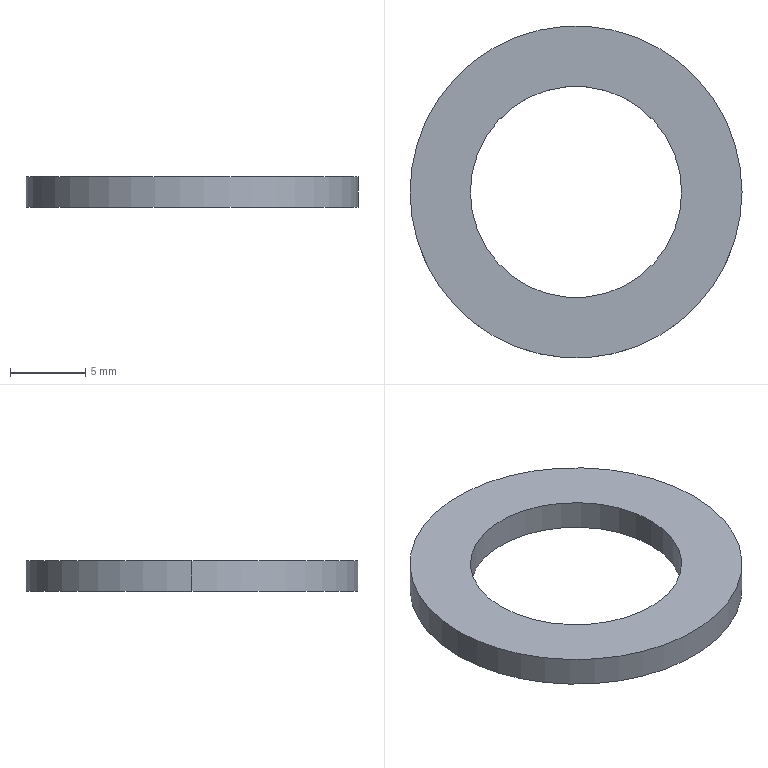Part | SolidWorks | features Extrusion 1 | 1 solid | 6 faces | box 22 x 22 x 2 mm | volume 452.389 mm3 | cylinder 4 | plane 2 | commonest cylinder face diameters 14 x2 22 x2
STEP:
#1=CARTESIAN_POINT('',(-7.,0.,2.));
#2=VERTEX_POINT('',#1);
#3=CARTESIAN_POINT('',(7.,0.,2.));
#4=VERTEX_POINT('',#3);
#5=CARTESIAN_POINT('',(0.,0.,2.));
#6=DIRECTION('',(0.,0.,1.));
#7=DIRECTION('',(1.,0.,0.));
#8=AXIS2_PLACEMENT_3D('',#5,#6,#7);
#9=CIRCLE('',#8,7.);
#10=EDGE_CURVE('',#2,#4,#9,.T.);
#11=ORIENTED_EDGE('',*,*,#10,.T.);
#12=CARTESIAN_POINT('',(7.,0.,0.));
#13=VERTEX_POINT('',#12);
#14=CARTESIAN_POINT('',(7.,0.,2.));
#15=DIRECTION('',(0.,0.,-1.));
#16=VECTOR('',#15,1000.);
#17=LINE('',#14,#16);
#18=EDGE_CURVE('',#4,#13,#17,.T.);
#19=ORIENTED_EDGE('',*,*,#18,.T.);
#20=CARTESIAN_POINT('',(-7.,0.,0.));
#21=VERTEX_POINT('',#20);
#22=CARTESIAN_POINT('',(0.,0.,0.));
#23=DIRECTION('',(0.,0.,1.));
#24=DIRECTION('',(1.,0.,0.));
#25=AXIS2_PLACEMENT_3D('',#22,#23,#24);
#26=CIRCLE('',#25,7.);
#27=EDGE_CURVE('',#21,#13,#26,.T.);
#28=ORIENTED_EDGE('',*,*,#27,.F.);
#29=CARTESIAN_POINT('',(-7.,0.,2.));
#30=DIRECTION('',(0.,0.,-1.));
#31=VECTOR('',#30,1000.);
#32=LINE('',#29,#31);
#33=EDGE_CURVE('',#2,#21,#32,.T.);
#34=ORIENTED_EDGE('',*,*,#33,.F.);
#35=EDGE_LOOP('',(#11,#19,#28,#34));
#36=FACE_OUTER_BOUND('',#35,.T.);
#37=CARTESIAN_POINT('',(0.,0.,2.));
#38=DIRECTION('',(0.,0.,-1.));
#39=DIRECTION('',(-1.,0.,0.));
#40=AXIS2_PLACEMENT_3D('',#37,#38,#39);
#41=CYLINDRICAL_SURFACE('',#40,7.);
#42=ADVANCED_FACE('',(#36),#41,.F.);
#43=CARTESIAN_POINT('',(11.,0.,2.));
#44=VERTEX_POINT('',#43);
#45=CARTESIAN_POINT('',(-11.,0.,2.));
#46=VERTEX_POINT('',#45);
#47=CARTESIAN_POINT('',(0.,0.,2.));
#48=DIRECTION('',(0.,0.,1.));
#49=DIRECTION('',(1.,0.,0.));
#50=AXIS2_PLACEMENT_3D('',#47,#48,#49);
#51=CIRCLE('',#50,11.);
#52=EDGE_CURVE('',#44,#46,#51,.T.);
#53=ORIENTED_EDGE('',*,*,#52,.F.);
#54=CARTESIAN_POINT('',(11.,0.,0.));
#55=VERTEX_POINT('',#54);
#56=CARTESIAN_POINT('',(11.,0.,2.));
#57=DIRECTION('',(0.,0.,-1.));
#58=VECTOR('',#57,1000.);
#59=LINE('',#56,#58);
#60=EDGE_CURVE('',#44,#55,#59,.T.);
#61=ORIENTED_EDGE('',*,*,#60,.T.);
#62=CARTESIAN_POINT('',(-11.,0.,0.));
#63=VERTEX_POINT('',#62);
#64=CARTESIAN_POINT('',(0.,0.,0.));
#65=DIRECTION('',(0.,0.,1.));
#66=DIRECTION('',(1.,0.,0.));
#67=AXIS2_PLACEMENT_3D('',#64,#65,#66);
#68=CIRCLE('',#67,11.);
#69=EDGE_CURVE('',#55,#63,#68,.T.);
#70=ORIENTED_EDGE('',*,*,#69,.T.);
#71=CARTESIAN_POINT('',(-11.,0.,2.));
#72=DIRECTION('',(0.,0.,-1.));
#73=VECTOR('',#72,1000.);
#74=LINE('',#71,#73);
#75=EDGE_CURVE('',#46,#63,#74,.T.);
#76=ORIENTED_EDGE('',*,*,#75,.F.);
#77=EDGE_LOOP('',(#53,#61,#70,#76));
#78=FACE_OUTER_BOUND('',#77,.T.);
#79=CARTESIAN_POINT('',(0.,0.,2.));
#80=DIRECTION('',(0.,0.,-1.));
#81=DIRECTION('',(-1.,0.,0.));
#82=AXIS2_PLACEMENT_3D('',#79,#80,#81);
#83=CYLINDRICAL_SURFACE('',#82,11.);
#84=ADVANCED_FACE('',(#78),#83,.T.);
#85=CARTESIAN_POINT('',(0.,0.,2.));
#86=DIRECTION('',(0.,0.,1.));
#87=DIRECTION('',(1.,0.,0.));
#88=AXIS2_PLACEMENT_3D('',#85,#86,#87);
#89=CIRCLE('',#88,11.);
#90=EDGE_CURVE('',#46,#44,#89,.T.);
#91=ORIENTED_EDGE('',*,*,#90,.T.);
#92=ORIENTED_EDGE('',*,*,#52,.T.);
#93=EDGE_LOOP('',(#91,#92));
#94=FACE_OUTER_BOUND('',#93,.T.);
#95=ORIENTED_EDGE('',*,*,#10,.F.);
#96=CARTESIAN_POINT('',(0.,0.,2.));
#97=DIRECTION('',(0.,0.,1.));
#98=DIRECTION('',(1.,0.,0.));
#99=AXIS2_PLACEMENT_3D('',#96,#97,#98);
#100=CIRCLE('',#99,7.);
#101=EDGE_CURVE('',#4,#2,#100,.T.);
#102=ORIENTED_EDGE('',*,*,#101,.F.);
#103=EDGE_LOOP('',(#95,#102));
#104=FACE_BOUND('',#103,.T.);
#105=CARTESIAN_POINT('',(0.,0.,2.));
#106=DIRECTION('',(0.,0.,1.));
#107=DIRECTION('',(1.,0.,0.));
#108=AXIS2_PLACEMENT_3D('',#105,#106,#107);
#109=PLANE('',#108);
#110=ADVANCED_FACE('',(#94,#104),#109,.T.);
#111=CARTESIAN_POINT('',(0.,0.,0.));
#112=DIRECTION('',(0.,0.,1.));
#113=DIRECTION('',(1.,0.,0.));
#114=AXIS2_PLACEMENT_3D('',#111,#112,#113);
#115=CIRCLE('',#114,11.);
#116=EDGE_CURVE('',#63,#55,#115,.T.);
#117=ORIENTED_EDGE('',*,*,#116,.F.);
#118=ORIENTED_EDGE('',*,*,#69,.F.);
#119=EDGE_LOOP('',(#117,#118));
#120=FACE_OUTER_BOUND('',#119,.T.);
#121=ORIENTED_EDGE('',*,*,#27,.T.);
#122=CARTESIAN_POINT('',(0.,0.,0.));
#123=DIRECTION('',(0.,0.,1.));
#124=DIRECTION('',(1.,0.,0.));
#125=AXIS2_PLACEMENT_3D('',#122,#123,#124);
#126=CIRCLE('',#125,7.);
#127=EDGE_CURVE('',#13,#21,#126,.T.);
#128=ORIENTED_EDGE('',*,*,#127,.T.);
#129=EDGE_LOOP('',(#121,#128));
#130=FACE_BOUND('',#129,.T.);
#131=CARTESIAN_POINT('',(0.,0.,0.));
#132=DIRECTION('',(0.,0.,1.));
#133=DIRECTION('',(1.,0.,0.));
#134=AXIS2_PLACEMENT_3D('',#131,#132,#133);
#135=PLANE('',#134);
#136=ADVANCED_FACE('',(#120,#130),#135,.F.);
#137=ORIENTED_EDGE('',*,*,#60,.F.);
#138=ORIENTED_EDGE('',*,*,#90,.F.);
#139=ORIENTED_EDGE('',*,*,#75,.T.);
#140=ORIENTED_EDGE('',*,*,#116,.T.);
#141=EDGE_LOOP('',(#137,#138,#139,#140));
#142=FACE_OUTER_BOUND('',#141,.T.);
#143=CARTESIAN_POINT('',(0.,0.,2.));
#144=DIRECTION('',(0.,0.,-1.));
#145=DIRECTION('',(-1.,0.,0.));
#146=AXIS2_PLACEMENT_3D('',#143,#144,#145);
#147=CYLINDRICAL_SURFACE('',#146,11.);
#148=ADVANCED_FACE('',(#142),#147,.T.);
#149=ORIENTED_EDGE('',*,*,#18,.F.);
#150=ORIENTED_EDGE('',*,*,#101,.T.);
#151=ORIENTED_EDGE('',*,*,#33,.T.);
#152=ORIENTED_EDGE('',*,*,#127,.F.);
#153=EDGE_LOOP('',(#149,#150,#151,#152));
#154=FACE_OUTER_BOUND('',#153,.T.);
#155=CARTESIAN_POINT('',(0.,0.,2.));
#156=DIRECTION('',(0.,0.,-1.));
#157=DIRECTION('',(-1.,0.,0.));
#158=AXIS2_PLACEMENT_3D('',#155,#156,#157);
#159=CYLINDRICAL_SURFACE('',#158,7.);
#160=ADVANCED_FACE('',(#154),#159,.F.);
#161=CLOSED_SHELL('',(#42,#84,#110,#136,#148,#160));
#162=MANIFOLD_SOLID_BREP('',#161);
#163=CARTESIAN_POINT('',(0.,0.,0.));
#164=DIRECTION('',(0.,0.,1.));
#165=DIRECTION('',(1.,0.,0.));
#166=AXIS2_PLACEMENT_3D('',#163,#164,#165);
#167=(LENGTH_UNIT()NAMED_UNIT(*)SI_UNIT(.MILLI.,.METRE.));
#168=UNCERTAINTY_MEASURE_WITH_UNIT(LENGTH_MEASURE(0.00001),#167,'','');
#169=(NAMED_UNIT(*)PLANE_ANGLE_UNIT()SI_UNIT($,.RADIAN.));
#170=(NAMED_UNIT(*)SI_UNIT($,.STERADIAN.)SOLID_ANGLE_UNIT());
#171=(GEOMETRIC_REPRESENTATION_CONTEXT(3)GLOBAL_UNCERTAINTY_ASSIGNED_CONTEXT((#168))GLOBAL_UNIT_ASSIGNED_CONTEXT((#167,#169,#170))REPRESENTATION_CONTEXT('',''));
#172=ADVANCED_BREP_SHAPE_REPRESENTATION('',(#162,#166),#171);